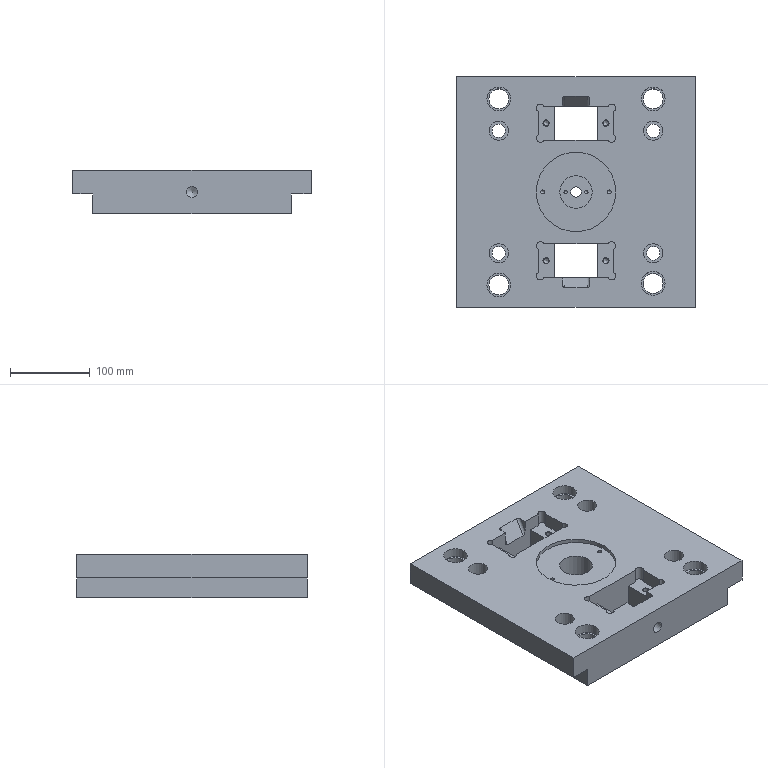Part | STEP file | AD_id274_x_t | 1 solid | 134 faces | box 300 x 290 x 55 mm | volume 3688496 mm3 | plane 59 | cylinder 53 | cone 22 | commonest cylinder face diameters 6.8 x8 10 x8 6 x4 7 x4 17 x4 24 x4